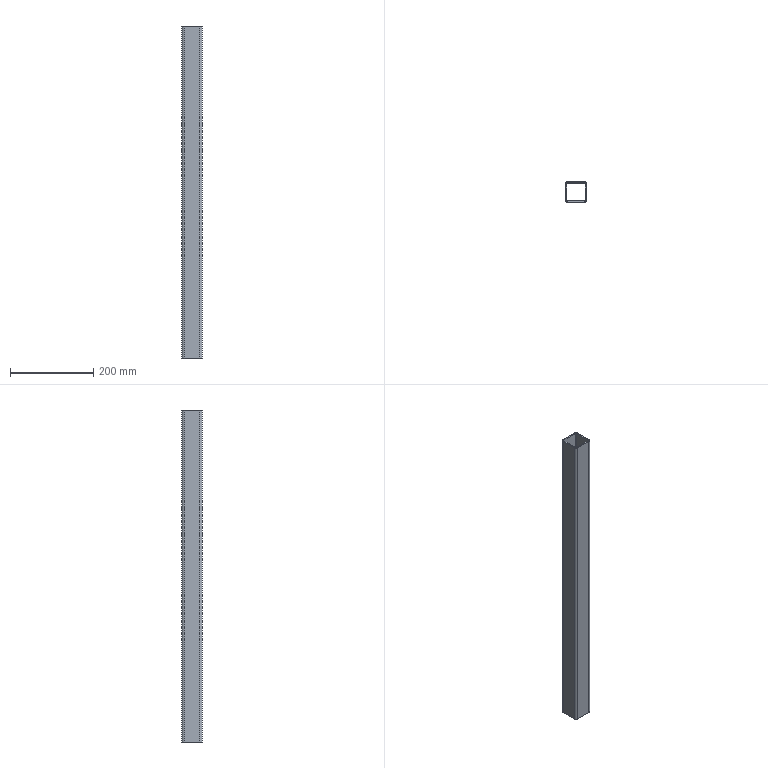Part | SolidWorks | 1 solid | 18 faces | box 50 x 50 x 800 mm | volume 432658 mm3 | plane 10 | cylinder 8 | commonest cylinder face diameters 6 x4 12 x4
STEP:
#1=CARTESIAN_POINT('',(19.,25.,400.));
#2=VERTEX_POINT('',#1);
#3=CARTESIAN_POINT('',(25.,19.,400.));
#4=VERTEX_POINT('',#3);
#5=CARTESIAN_POINT('',(19.,19.,400.));
#6=DIRECTION('',(0.,0.,-1.));
#7=DIRECTION('',(-1.,0.,0.));
#8=AXIS2_PLACEMENT_3D('',#5,#6,#7);
#9=CIRCLE('',#8,6.);
#10=EDGE_CURVE('',#2,#4,#9,.T.);
#11=ORIENTED_EDGE('',*,*,#10,.T.);
#12=CARTESIAN_POINT('',(25.,19.,-400.));
#13=VERTEX_POINT('',#12);
#14=CARTESIAN_POINT('',(25.,19.,-400.));
#15=DIRECTION('',(0.,0.,1.));
#16=VECTOR('',#15,1000.);
#17=LINE('',#14,#16);
#18=EDGE_CURVE('',#13,#4,#17,.T.);
#19=ORIENTED_EDGE('',*,*,#18,.F.);
#20=CARTESIAN_POINT('',(19.,25.,-400.));
#21=VERTEX_POINT('',#20);
#22=CARTESIAN_POINT('',(19.,19.,-400.));
#23=DIRECTION('',(0.,0.,-1.));
#24=DIRECTION('',(-1.,0.,0.));
#25=AXIS2_PLACEMENT_3D('',#22,#23,#24);
#26=CIRCLE('',#25,6.);
#27=EDGE_CURVE('',#21,#13,#26,.T.);
#28=ORIENTED_EDGE('',*,*,#27,.F.);
#29=CARTESIAN_POINT('',(19.,25.,-400.));
#30=DIRECTION('',(0.,0.,1.));
#31=VECTOR('',#30,1000.);
#32=LINE('',#29,#31);
#33=EDGE_CURVE('',#21,#2,#32,.T.);
#34=ORIENTED_EDGE('',*,*,#33,.T.);
#35=EDGE_LOOP('',(#11,#19,#28,#34));
#36=FACE_OUTER_BOUND('',#35,.T.);
#37=CARTESIAN_POINT('',(19.,19.,-400.));
#38=DIRECTION('',(0.,0.,1.));
#39=DIRECTION('',(1.,0.,0.));
#40=AXIS2_PLACEMENT_3D('',#37,#38,#39);
#41=CYLINDRICAL_SURFACE('',#40,6.);
#42=ADVANCED_FACE('',(#36),#41,.T.);
#43=CARTESIAN_POINT('',(25.,-19.,400.));
#44=VERTEX_POINT('',#43);
#45=CARTESIAN_POINT('',(25.,19.,400.));
#46=DIRECTION('',(0.,-1.,0.));
#47=VECTOR('',#46,1000.);
#48=LINE('',#45,#47);
#49=EDGE_CURVE('',#4,#44,#48,.T.);
#50=ORIENTED_EDGE('',*,*,#49,.T.);
#51=CARTESIAN_POINT('',(25.,-19.,-400.));
#52=VERTEX_POINT('',#51);
#53=CARTESIAN_POINT('',(25.,-19.,-400.));
#54=DIRECTION('',(0.,0.,1.));
#55=VECTOR('',#54,1000.);
#56=LINE('',#53,#55);
#57=EDGE_CURVE('',#52,#44,#56,.T.);
#58=ORIENTED_EDGE('',*,*,#57,.F.);
#59=CARTESIAN_POINT('',(25.,19.,-400.));
#60=DIRECTION('',(0.,-1.,0.));
#61=VECTOR('',#60,1000.);
#62=LINE('',#59,#61);
#63=EDGE_CURVE('',#13,#52,#62,.T.);
#64=ORIENTED_EDGE('',*,*,#63,.F.);
#65=ORIENTED_EDGE('',*,*,#18,.T.);
#66=EDGE_LOOP('',(#50,#58,#64,#65));
#67=FACE_OUTER_BOUND('',#66,.T.);
#68=CARTESIAN_POINT('',(25.,19.,-400.));
#69=DIRECTION('',(-1.,0.,0.));
#70=DIRECTION('',(0.,0.,1.));
#71=AXIS2_PLACEMENT_3D('',#68,#69,#70);
#72=PLANE('',#71);
#73=ADVANCED_FACE('',(#67),#72,.F.);
#74=CARTESIAN_POINT('',(19.,-25.,400.));
#75=VERTEX_POINT('',#74);
#76=CARTESIAN_POINT('',(19.,-19.,400.));
#77=DIRECTION('',(0.,0.,-1.));
#78=DIRECTION('',(-1.,0.,0.));
#79=AXIS2_PLACEMENT_3D('',#76,#77,#78);
#80=CIRCLE('',#79,6.);
#81=EDGE_CURVE('',#44,#75,#80,.T.);
#82=ORIENTED_EDGE('',*,*,#81,.T.);
#83=CARTESIAN_POINT('',(19.,-25.,-400.));
#84=VERTEX_POINT('',#83);
#85=CARTESIAN_POINT('',(19.,-25.,-400.));
#86=DIRECTION('',(0.,0.,1.));
#87=VECTOR('',#86,1000.);
#88=LINE('',#85,#87);
#89=EDGE_CURVE('',#84,#75,#88,.T.);
#90=ORIENTED_EDGE('',*,*,#89,.F.);
#91=CARTESIAN_POINT('',(19.,-19.,-400.));
#92=DIRECTION('',(0.,0.,-1.));
#93=DIRECTION('',(-1.,0.,0.));
#94=AXIS2_PLACEMENT_3D('',#91,#92,#93);
#95=CIRCLE('',#94,6.);
#96=EDGE_CURVE('',#52,#84,#95,.T.);
#97=ORIENTED_EDGE('',*,*,#96,.F.);
#98=ORIENTED_EDGE('',*,*,#57,.T.);
#99=EDGE_LOOP('',(#82,#90,#97,#98));
#100=FACE_OUTER_BOUND('',#99,.T.);
#101=CARTESIAN_POINT('',(19.,-19.,-400.));
#102=DIRECTION('',(0.,0.,1.));
#103=DIRECTION('',(1.,0.,0.));
#104=AXIS2_PLACEMENT_3D('',#101,#102,#103);
#105=CYLINDRICAL_SURFACE('',#104,6.);
#106=ADVANCED_FACE('',(#100),#105,.T.);
#107=CARTESIAN_POINT('',(-19.,-25.,400.));
#108=VERTEX_POINT('',#107);
#109=CARTESIAN_POINT('',(-19.,-25.,400.));
#110=DIRECTION('',(-1.,0.,0.));
#111=VECTOR('',#110,1000.);
#112=LINE('',#109,#111);
#113=EDGE_CURVE('',#75,#108,#112,.T.);
#114=ORIENTED_EDGE('',*,*,#113,.T.);
#115=CARTESIAN_POINT('',(-19.,-25.,-400.));
#116=VERTEX_POINT('',#115);
#117=CARTESIAN_POINT('',(-19.,-25.,-400.));
#118=DIRECTION('',(0.,0.,1.));
#119=VECTOR('',#118,1000.);
#120=LINE('',#117,#119);
#121=EDGE_CURVE('',#116,#108,#120,.T.);
#122=ORIENTED_EDGE('',*,*,#121,.F.);
#123=CARTESIAN_POINT('',(-19.,-25.,-400.));
#124=DIRECTION('',(-1.,0.,0.));
#125=VECTOR('',#124,1000.);
#126=LINE('',#123,#125);
#127=EDGE_CURVE('',#84,#116,#126,.T.);
#128=ORIENTED_EDGE('',*,*,#127,.F.);
#129=ORIENTED_EDGE('',*,*,#89,.T.);
#130=EDGE_LOOP('',(#114,#122,#128,#129));
#131=FACE_OUTER_BOUND('',#130,.T.);
#132=CARTESIAN_POINT('',(-19.,-25.,-400.));
#133=DIRECTION('',(0.,1.,0.));
#134=DIRECTION('',(0.,0.,1.));
#135=AXIS2_PLACEMENT_3D('',#132,#133,#134);
#136=PLANE('',#135);
#137=ADVANCED_FACE('',(#131),#136,.F.);
#138=CARTESIAN_POINT('',(-25.,-19.,400.));
#139=VERTEX_POINT('',#138);
#140=CARTESIAN_POINT('',(-19.,-19.,400.));
#141=DIRECTION('',(0.,0.,-1.));
#142=DIRECTION('',(-1.,0.,0.));
#143=AXIS2_PLACEMENT_3D('',#140,#141,#142);
#144=CIRCLE('',#143,6.);
#145=EDGE_CURVE('',#108,#139,#144,.T.);
#146=ORIENTED_EDGE('',*,*,#145,.T.);
#147=CARTESIAN_POINT('',(-25.,-19.,-400.));
#148=VERTEX_POINT('',#147);
#149=CARTESIAN_POINT('',(-25.,-19.,-400.));
#150=DIRECTION('',(0.,0.,1.));
#151=VECTOR('',#150,1000.);
#152=LINE('',#149,#151);
#153=EDGE_CURVE('',#148,#139,#152,.T.);
#154=ORIENTED_EDGE('',*,*,#153,.F.);
#155=CARTESIAN_POINT('',(-19.,-19.,-400.));
#156=DIRECTION('',(0.,0.,-1.));
#157=DIRECTION('',(-1.,0.,0.));
#158=AXIS2_PLACEMENT_3D('',#155,#156,#157);
#159=CIRCLE('',#158,6.);
#160=EDGE_CURVE('',#116,#148,#159,.T.);
#161=ORIENTED_EDGE('',*,*,#160,.F.);
#162=ORIENTED_EDGE('',*,*,#121,.T.);
#163=EDGE_LOOP('',(#146,#154,#161,#162));
#164=FACE_OUTER_BOUND('',#163,.T.);
#165=CARTESIAN_POINT('',(-19.,-19.,-400.));
#166=DIRECTION('',(0.,0.,1.));
#167=DIRECTION('',(1.,0.,0.));
#168=AXIS2_PLACEMENT_3D('',#165,#166,#167);
#169=CYLINDRICAL_SURFACE('',#168,6.);
#170=ADVANCED_FACE('',(#164),#169,.T.);
#171=CARTESIAN_POINT('',(-25.,19.,400.));
#172=VERTEX_POINT('',#171);
#173=CARTESIAN_POINT('',(-25.,-19.,400.));
#174=DIRECTION('',(0.,1.,0.));
#175=VECTOR('',#174,1000.);
#176=LINE('',#173,#175);
#177=EDGE_CURVE('',#139,#172,#176,.T.);
#178=ORIENTED_EDGE('',*,*,#177,.T.);
#179=CARTESIAN_POINT('',(-25.,19.,-400.));
#180=VERTEX_POINT('',#179);
#181=CARTESIAN_POINT('',(-25.,19.,-400.));
#182=DIRECTION('',(0.,0.,1.));
#183=VECTOR('',#182,1000.);
#184=LINE('',#181,#183);
#185=EDGE_CURVE('',#180,#172,#184,.T.);
#186=ORIENTED_EDGE('',*,*,#185,.F.);
#187=CARTESIAN_POINT('',(-25.,-19.,-400.));
#188=DIRECTION('',(0.,1.,0.));
#189=VECTOR('',#188,1000.);
#190=LINE('',#187,#189);
#191=EDGE_CURVE('',#148,#180,#190,.T.);
#192=ORIENTED_EDGE('',*,*,#191,.F.);
#193=ORIENTED_EDGE('',*,*,#153,.T.);
#194=EDGE_LOOP('',(#178,#186,#192,#193));
#195=FACE_OUTER_BOUND('',#194,.T.);
#196=CARTESIAN_POINT('',(-25.,-19.,-400.));
#197=DIRECTION('',(1.,0.,0.));
#198=DIRECTION('',(0.,0.,-1.));
#199=AXIS2_PLACEMENT_3D('',#196,#197,#198);
#200=PLANE('',#199);
#201=ADVANCED_FACE('',(#195),#200,.F.);
#202=CARTESIAN_POINT('',(-19.,25.,400.));
#203=VERTEX_POINT('',#202);
#204=CARTESIAN_POINT('',(-19.,19.,400.));
#205=DIRECTION('',(0.,0.,-1.));
#206=DIRECTION('',(-1.,0.,0.));
#207=AXIS2_PLACEMENT_3D('',#204,#205,#206);
#208=CIRCLE('',#207,6.);
#209=EDGE_CURVE('',#172,#203,#208,.T.);
#210=ORIENTED_EDGE('',*,*,#209,.T.);
#211=CARTESIAN_POINT('',(-19.,25.,-400.));
#212=VERTEX_POINT('',#211);
#213=CARTESIAN_POINT('',(-19.,25.,-400.));
#214=DIRECTION('',(0.,0.,1.));
#215=VECTOR('',#214,1000.);
#216=LINE('',#213,#215);
#217=EDGE_CURVE('',#212,#203,#216,.T.);
#218=ORIENTED_EDGE('',*,*,#217,.F.);
#219=CARTESIAN_POINT('',(-19.,19.,-400.));
#220=DIRECTION('',(0.,0.,-1.));
#221=DIRECTION('',(-1.,0.,0.));
#222=AXIS2_PLACEMENT_3D('',#219,#220,#221);
#223=CIRCLE('',#222,6.);
#224=EDGE_CURVE('',#180,#212,#223,.T.);
#225=ORIENTED_EDGE('',*,*,#224,.F.);
#226=ORIENTED_EDGE('',*,*,#185,.T.);
#227=EDGE_LOOP('',(#210,#218,#225,#226));
#228=FACE_OUTER_BOUND('',#227,.T.);
#229=CARTESIAN_POINT('',(-19.,19.,-400.));
#230=DIRECTION('',(0.,0.,1.));
#231=DIRECTION('',(1.,0.,0.));
#232=AXIS2_PLACEMENT_3D('',#229,#230,#231);
#233=CYLINDRICAL_SURFACE('',#232,6.);
#234=ADVANCED_FACE('',(#228),#233,.T.);
#235=CARTESIAN_POINT('',(22.,-19.,400.));
#236=VERTEX_POINT('',#235);
#237=CARTESIAN_POINT('',(19.,-22.,400.));
#238=VERTEX_POINT('',#237);
#239=CARTESIAN_POINT('',(19.,-19.,400.));
#240=DIRECTION('',(0.,0.,-1.));
#241=DIRECTION('',(-1.,0.,0.));
#242=AXIS2_PLACEMENT_3D('',#239,#240,#241);
#243=CIRCLE('',#242,3.);
#244=EDGE_CURVE('',#236,#238,#243,.T.);
#245=ORIENTED_EDGE('',*,*,#244,.F.);
#246=CARTESIAN_POINT('',(22.,-19.,-400.));
#247=VERTEX_POINT('',#246);
#248=CARTESIAN_POINT('',(22.,-19.,-400.));
#249=DIRECTION('',(0.,0.,1.));
#250=VECTOR('',#249,1000.);
#251=LINE('',#248,#250);
#252=EDGE_CURVE('',#247,#236,#251,.T.);
#253=ORIENTED_EDGE('',*,*,#252,.F.);
#254=CARTESIAN_POINT('',(19.,-22.,-400.));
#255=VERTEX_POINT('',#254);
#256=CARTESIAN_POINT('',(19.,-19.,-400.));
#257=DIRECTION('',(0.,0.,-1.));
#258=DIRECTION('',(-1.,0.,0.));
#259=AXIS2_PLACEMENT_3D('',#256,#257,#258);
#260=CIRCLE('',#259,3.);
#261=EDGE_CURVE('',#247,#255,#260,.T.);
#262=ORIENTED_EDGE('',*,*,#261,.T.);
#263=CARTESIAN_POINT('',(19.,-22.,-400.));
#264=DIRECTION('',(0.,0.,1.));
#265=VECTOR('',#264,1000.);
#266=LINE('',#263,#265);
#267=EDGE_CURVE('',#255,#238,#266,.T.);
#268=ORIENTED_EDGE('',*,*,#267,.T.);
#269=EDGE_LOOP('',(#245,#253,#262,#268));
#270=FACE_OUTER_BOUND('',#269,.T.);
#271=CARTESIAN_POINT('',(19.,-19.,-400.));
#272=DIRECTION('',(0.,0.,1.));
#273=DIRECTION('',(1.,0.,0.));
#274=AXIS2_PLACEMENT_3D('',#271,#272,#273);
#275=CYLINDRICAL_SURFACE('',#274,3.);
#276=ADVANCED_FACE('',(#270),#275,.F.);
#277=CARTESIAN_POINT('',(22.,19.,400.));
#278=VERTEX_POINT('',#277);
#279=CARTESIAN_POINT('',(22.,19.,400.));
#280=DIRECTION('',(0.,-1.,0.));
#281=VECTOR('',#280,1000.);
#282=LINE('',#279,#281);
#283=EDGE_CURVE('',#278,#236,#282,.T.);
#284=ORIENTED_EDGE('',*,*,#283,.F.);
#285=CARTESIAN_POINT('',(22.,19.,-400.));
#286=VERTEX_POINT('',#285);
#287=CARTESIAN_POINT('',(22.,19.,-400.));
#288=DIRECTION('',(0.,0.,1.));
#289=VECTOR('',#288,1000.);
#290=LINE('',#287,#289);
#291=EDGE_CURVE('',#286,#278,#290,.T.);
#292=ORIENTED_EDGE('',*,*,#291,.F.);
#293=CARTESIAN_POINT('',(22.,19.,-400.));
#294=DIRECTION('',(0.,-1.,0.));
#295=VECTOR('',#294,1000.);
#296=LINE('',#293,#295);
#297=EDGE_CURVE('',#286,#247,#296,.T.);
#298=ORIENTED_EDGE('',*,*,#297,.T.);
#299=ORIENTED_EDGE('',*,*,#252,.T.);
#300=EDGE_LOOP('',(#284,#292,#298,#299));
#301=FACE_OUTER_BOUND('',#300,.T.);
#302=CARTESIAN_POINT('',(22.,19.,-400.));
#303=DIRECTION('',(-1.,0.,0.));
#304=DIRECTION('',(0.,0.,1.));
#305=AXIS2_PLACEMENT_3D('',#302,#303,#304);
#306=PLANE('',#305);
#307=ADVANCED_FACE('',(#301),#306,.T.);
#308=CARTESIAN_POINT('',(19.,22.,400.));
#309=VERTEX_POINT('',#308);
#310=CARTESIAN_POINT('',(19.,19.,400.));
#311=DIRECTION('',(0.,0.,-1.));
#312=DIRECTION('',(-1.,0.,0.));
#313=AXIS2_PLACEMENT_3D('',#310,#311,#312);
#314=CIRCLE('',#313,3.);
#315=EDGE_CURVE('',#309,#278,#314,.T.);
#316=ORIENTED_EDGE('',*,*,#315,.F.);
#317=CARTESIAN_POINT('',(19.,22.,-400.));
#318=VERTEX_POINT('',#317);
#319=CARTESIAN_POINT('',(19.,22.,-400.));
#320=DIRECTION('',(0.,0.,1.));
#321=VECTOR('',#320,1000.);
#322=LINE('',#319,#321);
#323=EDGE_CURVE('',#318,#309,#322,.T.);
#324=ORIENTED_EDGE('',*,*,#323,.F.);
#325=CARTESIAN_POINT('',(19.,19.,-400.));
#326=DIRECTION('',(0.,0.,-1.));
#327=DIRECTION('',(-1.,0.,0.));
#328=AXIS2_PLACEMENT_3D('',#325,#326,#327);
#329=CIRCLE('',#328,3.);
#330=EDGE_CURVE('',#318,#286,#329,.T.);
#331=ORIENTED_EDGE('',*,*,#330,.T.);
#332=ORIENTED_EDGE('',*,*,#291,.T.);
#333=EDGE_LOOP('',(#316,#324,#331,#332));
#334=FACE_OUTER_BOUND('',#333,.T.);
#335=CARTESIAN_POINT('',(19.,19.,-400.));
#336=DIRECTION('',(0.,0.,1.));
#337=DIRECTION('',(1.,0.,0.));
#338=AXIS2_PLACEMENT_3D('',#335,#336,#337);
#339=CYLINDRICAL_SURFACE('',#338,3.);
#340=ADVANCED_FACE('',(#334),#339,.F.);
#341=CARTESIAN_POINT('',(-19.,22.,400.));
#342=VERTEX_POINT('',#341);
#343=CARTESIAN_POINT('',(19.,22.,400.));
#344=DIRECTION('',(1.,0.,0.));
#345=VECTOR('',#344,1000.);
#346=LINE('',#343,#345);
#347=EDGE_CURVE('',#342,#309,#346,.T.);
#348=ORIENTED_EDGE('',*,*,#347,.F.);
#349=CARTESIAN_POINT('',(-19.,22.,-400.));
#350=VERTEX_POINT('',#349);
#351=CARTESIAN_POINT('',(-19.,22.,-400.));
#352=DIRECTION('',(0.,0.,1.));
#353=VECTOR('',#352,1000.);
#354=LINE('',#351,#353);
#355=EDGE_CURVE('',#350,#342,#354,.T.);
#356=ORIENTED_EDGE('',*,*,#355,.F.);
#357=CARTESIAN_POINT('',(19.,22.,-400.));
#358=DIRECTION('',(1.,0.,0.));
#359=VECTOR('',#358,1000.);
#360=LINE('',#357,#359);
#361=EDGE_CURVE('',#350,#318,#360,.T.);
#362=ORIENTED_EDGE('',*,*,#361,.T.);
#363=ORIENTED_EDGE('',*,*,#323,.T.);
#364=EDGE_LOOP('',(#348,#356,#362,#363));
#365=FACE_OUTER_BOUND('',#364,.T.);
#366=CARTESIAN_POINT('',(19.,22.,-400.));
#367=DIRECTION('',(0.,-1.,0.));
#368=DIRECTION('',(0.,0.,-1.));
#369=AXIS2_PLACEMENT_3D('',#366,#367,#368);
#370=PLANE('',#369);
#371=ADVANCED_FACE('',(#365),#370,.T.);
#372=CARTESIAN_POINT('',(-22.,19.,400.));
#373=VERTEX_POINT('',#372);
#374=CARTESIAN_POINT('',(-19.,19.,400.));
#375=DIRECTION('',(0.,0.,-1.));
#376=DIRECTION('',(-1.,0.,0.));
#377=AXIS2_PLACEMENT_3D('',#374,#375,#376);
#378=CIRCLE('',#377,3.);
#379=EDGE_CURVE('',#373,#342,#378,.T.);
#380=ORIENTED_EDGE('',*,*,#379,.F.);
#381=CARTESIAN_POINT('',(-22.,19.,-400.));
#382=VERTEX_POINT('',#381);
#383=CARTESIAN_POINT('',(-22.,19.,-400.));
#384=DIRECTION('',(0.,0.,1.));
#385=VECTOR('',#384,1000.);
#386=LINE('',#383,#385);
#387=EDGE_CURVE('',#382,#373,#386,.T.);
#388=ORIENTED_EDGE('',*,*,#387,.F.);
#389=CARTESIAN_POINT('',(-19.,19.,-400.));
#390=DIRECTION('',(0.,0.,-1.));
#391=DIRECTION('',(-1.,0.,0.));
#392=AXIS2_PLACEMENT_3D('',#389,#390,#391);
#393=CIRCLE('',#392,3.);
#394=EDGE_CURVE('',#382,#350,#393,.T.);
#395=ORIENTED_EDGE('',*,*,#394,.T.);
#396=ORIENTED_EDGE('',*,*,#355,.T.);
#397=EDGE_LOOP('',(#380,#388,#395,#396));
#398=FACE_OUTER_BOUND('',#397,.T.);
#399=CARTESIAN_POINT('',(-19.,19.,-400.));
#400=DIRECTION('',(0.,0.,1.));
#401=DIRECTION('',(1.,0.,0.));
#402=AXIS2_PLACEMENT_3D('',#399,#400,#401);
#403=CYLINDRICAL_SURFACE('',#402,3.);
#404=ADVANCED_FACE('',(#398),#403,.F.);
#405=CARTESIAN_POINT('',(-22.,-19.,400.));
#406=VERTEX_POINT('',#405);
#407=CARTESIAN_POINT('',(-22.,-19.,400.));
#408=DIRECTION('',(0.,1.,0.));
#409=VECTOR('',#408,1000.);
#410=LINE('',#407,#409);
#411=EDGE_CURVE('',#406,#373,#410,.T.);
#412=ORIENTED_EDGE('',*,*,#411,.F.);
#413=CARTESIAN_POINT('',(-22.,-19.,-400.));
#414=VERTEX_POINT('',#413);
#415=CARTESIAN_POINT('',(-22.,-19.,-400.));
#416=DIRECTION('',(0.,0.,1.));
#417=VECTOR('',#416,1000.);
#418=LINE('',#415,#417);
#419=EDGE_CURVE('',#414,#406,#418,.T.);
#420=ORIENTED_EDGE('',*,*,#419,.F.);
#421=CARTESIAN_POINT('',(-22.,-19.,-400.));
#422=DIRECTION('',(0.,1.,0.));
#423=VECTOR('',#422,1000.);
#424=LINE('',#421,#423);
#425=EDGE_CURVE('',#414,#382,#424,.T.);
#426=ORIENTED_EDGE('',*,*,#425,.T.);
#427=ORIENTED_EDGE('',*,*,#387,.T.);
#428=EDGE_LOOP('',(#412,#420,#426,#427));
#429=FACE_OUTER_BOUND('',#428,.T.);
#430=CARTESIAN_POINT('',(-22.,-19.,-400.));
#431=DIRECTION('',(1.,0.,0.));
#432=DIRECTION('',(0.,0.,-1.));
#433=AXIS2_PLACEMENT_3D('',#430,#431,#432);
#434=PLANE('',#433);
#435=ADVANCED_FACE('',(#429),#434,.T.);
#436=CARTESIAN_POINT('',(-19.,-22.,400.));
#437=VERTEX_POINT('',#436);
#438=CARTESIAN_POINT('',(-19.,-19.,400.));
#439=DIRECTION('',(0.,0.,-1.));
#440=DIRECTION('',(-1.,0.,0.));
#441=AXIS2_PLACEMENT_3D('',#438,#439,#440);
#442=CIRCLE('',#441,3.);
#443=EDGE_CURVE('',#437,#406,#442,.T.);
#444=ORIENTED_EDGE('',*,*,#443,.F.);
#445=CARTESIAN_POINT('',(-19.,-22.,-400.));
#446=VERTEX_POINT('',#445);
#447=CARTESIAN_POINT('',(-19.,-22.,-400.));
#448=DIRECTION('',(0.,0.,1.));
#449=VECTOR('',#448,1000.);
#450=LINE('',#447,#449);
#451=EDGE_CURVE('',#446,#437,#450,.T.);
#452=ORIENTED_EDGE('',*,*,#451,.F.);
#453=CARTESIAN_POINT('',(-19.,-19.,-400.));
#454=DIRECTION('',(0.,0.,-1.));
#455=DIRECTION('',(-1.,0.,0.));
#456=AXIS2_PLACEMENT_3D('',#453,#454,#455);
#457=CIRCLE('',#456,3.);
#458=EDGE_CURVE('',#446,#414,#457,.T.);
#459=ORIENTED_EDGE('',*,*,#458,.T.);
#460=ORIENTED_EDGE('',*,*,#419,.T.);
#461=EDGE_LOOP('',(#444,#452,#459,#460));
#462=FACE_OUTER_BOUND('',#461,.T.);
#463=CARTESIAN_POINT('',(-19.,-19.,-400.));
#464=DIRECTION('',(0.,0.,1.));
#465=DIRECTION('',(1.,0.,0.));
#466=AXIS2_PLACEMENT_3D('',#463,#464,#465);
#467=CYLINDRICAL_SURFACE('',#466,3.);
#468=ADVANCED_FACE('',(#462),#467,.F.);
#469=CARTESIAN_POINT('',(-19.,-22.,400.));
#470=DIRECTION('',(-1.,0.,0.));
#471=VECTOR('',#470,1000.);
#472=LINE('',#469,#471);
#473=EDGE_CURVE('',#238,#437,#472,.T.);
#474=ORIENTED_EDGE('',*,*,#473,.F.);
#475=ORIENTED_EDGE('',*,*,#267,.F.);
#476=CARTESIAN_POINT('',(-19.,-22.,-400.));
#477=DIRECTION('',(-1.,0.,0.));
#478=VECTOR('',#477,1000.);
#479=LINE('',#476,#478);
#480=EDGE_CURVE('',#255,#446,#479,.T.);
#481=ORIENTED_EDGE('',*,*,#480,.T.);
#482=ORIENTED_EDGE('',*,*,#451,.T.);
#483=EDGE_LOOP('',(#474,#475,#481,#482));
#484=FACE_OUTER_BOUND('',#483,.T.);
#485=CARTESIAN_POINT('',(-19.,-22.,-400.));
#486=DIRECTION('',(0.,1.,0.));
#487=DIRECTION('',(0.,0.,1.));
#488=AXIS2_PLACEMENT_3D('',#485,#486,#487);
#489=PLANE('',#488);
#490=ADVANCED_FACE('',(#484),#489,.T.);
#491=CARTESIAN_POINT('',(19.,25.,400.));
#492=DIRECTION('',(1.,0.,0.));
#493=VECTOR('',#492,1000.);
#494=LINE('',#491,#493);
#495=EDGE_CURVE('',#203,#2,#494,.T.);
#496=ORIENTED_EDGE('',*,*,#495,.T.);
#497=ORIENTED_EDGE('',*,*,#33,.F.);
#498=CARTESIAN_POINT('',(19.,25.,-400.));
#499=DIRECTION('',(1.,0.,0.));
#500=VECTOR('',#499,1000.);
#501=LINE('',#498,#500);
#502=EDGE_CURVE('',#212,#21,#501,.T.);
#503=ORIENTED_EDGE('',*,*,#502,.F.);
#504=ORIENTED_EDGE('',*,*,#217,.T.);
#505=EDGE_LOOP('',(#496,#497,#503,#504));
#506=FACE_OUTER_BOUND('',#505,.T.);
#507=CARTESIAN_POINT('',(19.,25.,-400.));
#508=DIRECTION('',(0.,-1.,0.));
#509=DIRECTION('',(0.,0.,-1.));
#510=AXIS2_PLACEMENT_3D('',#507,#508,#509);
#511=PLANE('',#510);
#512=ADVANCED_FACE('',(#506),#511,.F.);
#513=ORIENTED_EDGE('',*,*,#261,.F.);
#514=ORIENTED_EDGE('',*,*,#297,.F.);
#515=ORIENTED_EDGE('',*,*,#330,.F.);
#516=ORIENTED_EDGE('',*,*,#361,.F.);
#517=ORIENTED_EDGE('',*,*,#394,.F.);
#518=ORIENTED_EDGE('',*,*,#425,.F.);
#519=ORIENTED_EDGE('',*,*,#458,.F.);
#520=ORIENTED_EDGE('',*,*,#480,.F.);
#521=EDGE_LOOP('',(#513,#514,#515,#516,#517,#518,#519,#520));
#522=FACE_BOUND('',#521,.T.);
#523=ORIENTED_EDGE('',*,*,#27,.T.);
#524=ORIENTED_EDGE('',*,*,#63,.T.);
#525=ORIENTED_EDGE('',*,*,#96,.T.);
#526=ORIENTED_EDGE('',*,*,#127,.T.);
#527=ORIENTED_EDGE('',*,*,#160,.T.);
#528=ORIENTED_EDGE('',*,*,#191,.T.);
#529=ORIENTED_EDGE('',*,*,#224,.T.);
#530=ORIENTED_EDGE('',*,*,#502,.T.);
#531=EDGE_LOOP('',(#523,#524,#525,#526,#527,#528,#529,#530));
#532=FACE_OUTER_BOUND('',#531,.T.);
#533=CARTESIAN_POINT('',(19.,19.,-400.));
#534=DIRECTION('',(0.,0.,-1.));
#535=DIRECTION('',(-1.,0.,0.));
#536=AXIS2_PLACEMENT_3D('',#533,#534,#535);
#537=PLANE('',#536);
#538=ADVANCED_FACE('',(#522,#532),#537,.T.);
#539=ORIENTED_EDGE('',*,*,#244,.T.);
#540=ORIENTED_EDGE('',*,*,#473,.T.);
#541=ORIENTED_EDGE('',*,*,#443,.T.);
#542=ORIENTED_EDGE('',*,*,#411,.T.);
#543=ORIENTED_EDGE('',*,*,#379,.T.);
#544=ORIENTED_EDGE('',*,*,#347,.T.);
#545=ORIENTED_EDGE('',*,*,#315,.T.);
#546=ORIENTED_EDGE('',*,*,#283,.T.);
#547=EDGE_LOOP('',(#539,#540,#541,#542,#543,#544,#545,#546));
#548=FACE_BOUND('',#547,.T.);
#549=ORIENTED_EDGE('',*,*,#10,.F.);
#550=ORIENTED_EDGE('',*,*,#495,.F.);
#551=ORIENTED_EDGE('',*,*,#209,.F.);
#552=ORIENTED_EDGE('',*,*,#177,.F.);
#553=ORIENTED_EDGE('',*,*,#145,.F.);
#554=ORIENTED_EDGE('',*,*,#113,.F.);
#555=ORIENTED_EDGE('',*,*,#81,.F.);
#556=ORIENTED_EDGE('',*,*,#49,.F.);
#557=EDGE_LOOP('',(#549,#550,#551,#552,#553,#554,#555,#556));
#558=FACE_OUTER_BOUND('',#557,.T.);
#559=CARTESIAN_POINT('',(19.,19.,400.));
#560=DIRECTION('',(0.,0.,-1.));
#561=DIRECTION('',(-1.,0.,0.));
#562=AXIS2_PLACEMENT_3D('',#559,#560,#561);
#563=PLANE('',#562);
#564=ADVANCED_FACE('',(#548,#558),#563,.F.);
#565=CLOSED_SHELL('',(#42,#73,#106,#137,#170,#201,#234,#276,#307,#340,#371,#404,#435,#468,#490,#512,#538,#564));
#566=MANIFOLD_SOLID_BREP('',#565);
#567=CARTESIAN_POINT('',(0.,0.,0.));
#568=DIRECTION('',(0.,0.,1.));
#569=DIRECTION('',(1.,0.,0.));
#570=AXIS2_PLACEMENT_3D('',#567,#568,#569);
#571=(LENGTH_UNIT()NAMED_UNIT(*)SI_UNIT(.MILLI.,.METRE.));
#572=UNCERTAINTY_MEASURE_WITH_UNIT(LENGTH_MEASURE(0.00001),#571,'','');
#573=(NAMED_UNIT(*)PLANE_ANGLE_UNIT()SI_UNIT($,.RADIAN.));
#574=(NAMED_UNIT(*)SI_UNIT($,.STERADIAN.)SOLID_ANGLE_UNIT());
#575=(GEOMETRIC_REPRESENTATION_CONTEXT(3)GLOBAL_UNCERTAINTY_ASSIGNED_CONTEXT((#572))GLOBAL_UNIT_ASSIGNED_CONTEXT((#571,#573,#574))REPRESENTATION_CONTEXT('',''));
#576=ADVANCED_BREP_SHAPE_REPRESENTATION('',(#566,#570),#575);